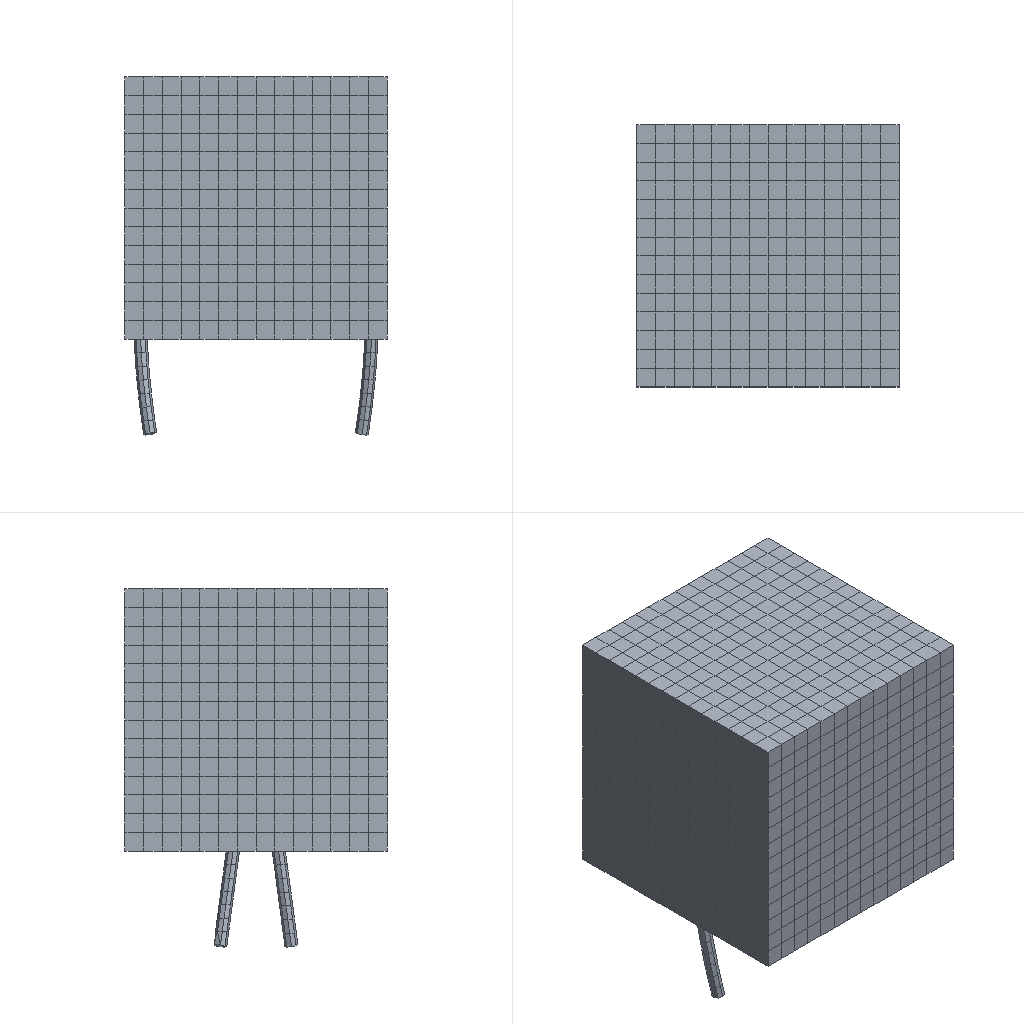Simulation study | abaqus
Set-up summary:
category,name,step,type,value,unit,region
solver,abaqus
solver,version,,,Abaqus/Standard 2020
units,not stated in the deck,,not stated
analysis,deck,,static,static
load_step,Step-1,Step-1,static
load_step,requested,,,1
mesh,nodes,,,4374
mesh,elements,,,3184
element_type,C3D8R,,solid,3184
load,load commands in deck,,count,1
bc,support commands in deck,,count,6
material,BASE,,in results
material,FIBER,,in results
check,setup vs results,,match,"per instance, exact: element labels, types and connectivity; labels of the nodes the elements use; coordinates of those nodes at SINGLE_PRECISION in 2 of 2 instance(s)"
Abaqus input file, long lists of numbers shortened:
*Heading
** Job name: Job-2 Model name: Model-1-Copy
** Generated by: Abaqus/CAE 2020
*Preprint, echo=NO, model=NO, history=NO, contact=NO
**
** PARTS
**
*Part, name=part-8
*End Part
**
*Part, name=part-12
*End Part
**
**
** ASSEMBLY
**
*Assembly, name=Assembly
**
*Instance, name=part-8-1, part=part-8
   -11.,     0.006016, -0.6108
*Node
      1,   11.857,   4.119,  0.6108
      2,   11.357,   4.129,  0.6108
** (997 more lines like these left out)
*Element, type=C3D8R
  1, 247,  11,  12,   2, 893, 535, 536, 205
  2, 247,   1,  10,  11, 893,  16, 534, 535
** (438 more lines like these left out)
*Nset, nset=Set-1, generate
   1,  999,    1
*Elset, elset=Set-1, generate
   1,  440,    1
** Section: fiber
*Solid Section, elset=Set-1, material=fiber
,
*End Instance
**
*Instance, name=part-12-1, part=part-12
*Node
      1,          10.,          10.,           0.
      2,   9.286,          10.,           0.
** (3373 more lines like these left out)
*Element, type=C3D8R
   1,  226,  227,  242,  241,    1,    2,   17,   16
   2,  227,  228,  243,  242,    2,    3,   18,   17
** (2742 more lines like these left out)
*Nset, nset=Set-1, generate
    1,  3375,     1
*Elset, elset=Set-1, generate
    1,  2744,     1
** Section: base
*Solid Section, elset=Set-1, material=base
,
*End Instance
**
*Nset, nset=Set-3, instance=part-12-1
    1,    2,    3,    4,    5,    6,    7,    8,    9,   10,   11,   12,   13,   14,   15,  226
  227,  228,  229,  230,  231,  232,  233,  234,  235,  236,  237,  238,  239,  240,  451,  452
** (13 more lines like these left out)
*Elset, elset=Set-3, instance=part-12-1
    1,    2,    3,    4,    5,    6,    7,    8,    9,   10,   11,   12,   13,   14,  197,  198
  199,  200,  201,  202,  203,  204,  205,  206,  207,  208,  209,  210,  393,  394,  395,  396
** (11 more lines like these left out)
*Nset, nset=Set-4, instance=part-12-1, generate
 3151,  3375,     1
*Elset, elset=Set-4, instance=part-12-1, generate
 2549,  2744,     1
*Nset, nset=Set-5, instance=part-12-1, generate
    1,  3361,    15
*Elset, elset=Set-5, instance=part-12-1, generate
    1,  2731,    14
*Nset, nset=Set-6, instance=part-12-1, generate
   15,  3375,    15
*Elset, elset=Set-6, instance=part-12-1, generate
   14,  2744,    14
*Nset, nset=m_Set-1, instance=part-8-1
   1,   2,   3,   4,  10,  11,  12,  13,  14,  15,  16,  17,  18,  19,  20,  21
  22,  23,  24,  25,  26,  27,  28,  29,  30,  31,  32,  33,  34,  35,  36,  37
** (53 more lines like these left out)
*Elset, elset=m_Set-1, instance=part-8-1, generate
   1,  384,    1
*Nset, nset=s_Set-1, instance=part-12-1, generate
    1,  3375,     1
*Elset, elset=s_Set-1, instance=part-12-1, generate
    1,  2744,     1
*Elset, elset=_Surf-1_S5, internal, instance=part-12-1
  183,  184,  185,  186,  187,  188,  189,  190,  191,  192,  193,  194,  195,  196,  379,  380
  381,  382,  383,  384,  385,  386,  387,  388,  389,  390,  391,  392,  575,  576,  577,  578
** (11 more lines like these left out)
*Surface, type=ELEMENT, name=Surf-1
_Surf-1_S5, S5
*Elset, elset=_Surf-2_S4, internal, instance=part-12-1, generate
   14,  2744,    14
*Surface, type=ELEMENT, name=Surf-2
_Surf-2_S4, S4
*Elset, elset=_Surf-3_S2, internal, instance=part-12-1, generate
   1,  196,    1
*Surface, type=ELEMENT, name=Surf-3
_Surf-3_S2, S2
*Elset, elset=_Surf-4_S6, internal, instance=part-12-1, generate
    1,  2731,    14
*Surface, type=ELEMENT, name=Surf-4
_Surf-4_S6, S6
** Constraint: Constraint-1
*Embedded Element, host elset=s_Set-1
m_Set-1
*End Assembly
*Amplitude, name=Amp-1
             0.,              0.,              1.,              1.
**
** MATERIALS
**
*Material, name=base
*Density
 1e-09,
*Elastic
 2.05, 0.47
*Material, name=fiber
*Density
 1.15e-09,
*Elastic
1590., 0.37
** ----------------------------------------------------------------
**
** STEP: Step-1
**
*Step, name=Step-1, nlgeom=YES, inc=1000
*Static, stabilize=0.0002, allsdtol=0.05, continue=NO
0.01, 1., 1e-05, 1.
**
** BOUNDARY CONDITIONS
**
** Name: BC-2 Type: 位移/转角
*Boundary
Set-6, 1, 1
Set-6, 2, 2
Set-6, 3, 3
Set-6, 4, 4
Set-6, 5, 5
Set-6, 6, 6
**
** LOADS
**
** Name: Load-3   Type: Pressure
*Dsload, amplitude=Amp-1
Surf-4, P, 0.1
**
** OUTPUT REQUESTS
**
*Restart, write, frequency=0
**
** FIELD OUTPUT: F-Output-1
**
*Output, field
*Node Output
CF, RF, U, V
*Element Output, directions=YES
E, LE, MISES, PE, PEEQ, PEMAG, S
*Contact Output
CDISP, CSTRESS
**
** HISTORY OUTPUT: H-Output-1
**
*Output, history, variable=PRESELECT
*End Step
Results summary:
result,step,,completed,increments=11 time=1.0/1.0
result,analysis,,,static
result,last_loadstep,,,1
result,primary field,,,U
result,reaction total,,FX,10.429,model units
result,reaction total,,FY,0.001069,model units
result,reaction total,,FZ,-0.0584,model units